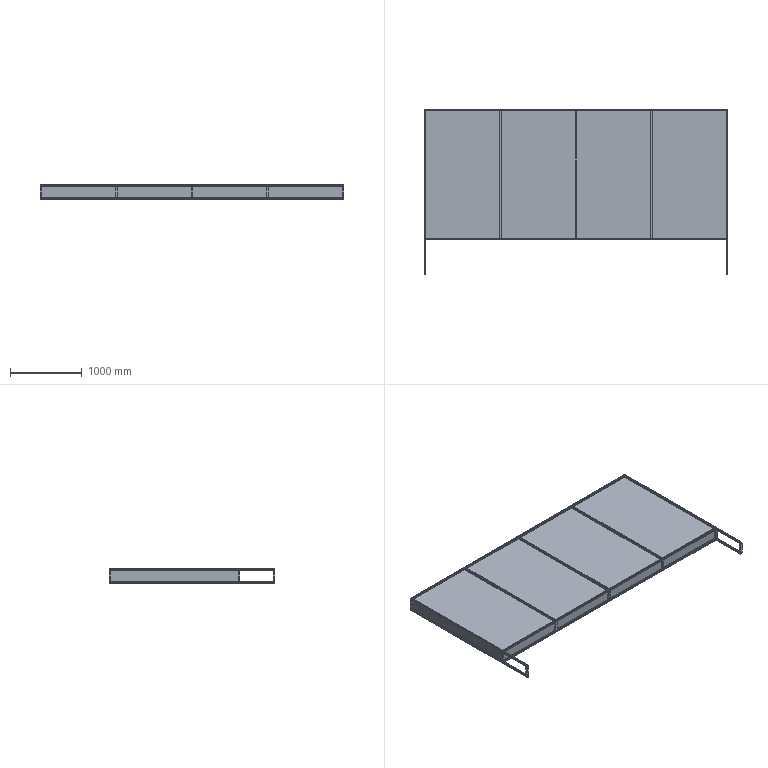Part | SolidWorks | features ICE 2, LPattern 2, WeldMemberFeat 1, WeldmentFeature 1 | 30 solids | 348 faces | box 4240 x 2313 x 200 mm | volume 1102421042 mm3 | plane 236 | cylinder 112 | commonest cylinder face diameters 3.5 x56 7 x56